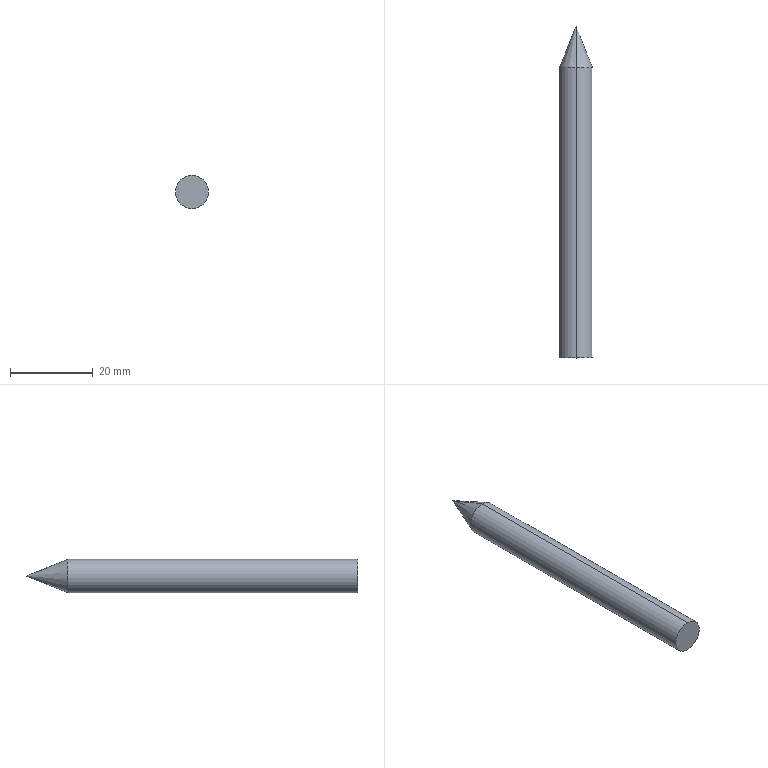Part | SolidWorks | features MirrorStock 1 | 1 solid | 5 faces | box 8 x 80 x 8 mm | volume 3686 mm3 | cone 2 | cylinder 2 | plane 1 | commonest cylinder face diameters 8 x2
STEP:
#1=CARTESIAN_POINT('',(0.,80.,0.));
#2=VERTEX_POINT('',#1);
#3=CARTESIAN_POINT('',(0.,70.,4.));
#4=VERTEX_POINT('',#3);
#5=CARTESIAN_POINT('',(0.,80.,0.));
#6=DIRECTION('',(0.,-0.9285,0.3714));
#7=VECTOR('',#6,1000.);
#8=LINE('',#5,#7);
#9=EDGE_CURVE('',#2,#4,#8,.T.);
#10=ORIENTED_EDGE('',*,*,#9,.F.);
#11=CARTESIAN_POINT('',(0.,70.,-4.));
#12=VERTEX_POINT('',#11);
#13=CARTESIAN_POINT('',(0.,80.,0.));
#14=DIRECTION('',(0.,-0.9285,-0.3714));
#15=VECTOR('',#14,1000.);
#16=LINE('',#13,#15);
#17=EDGE_CURVE('',#2,#12,#16,.T.);
#18=ORIENTED_EDGE('',*,*,#17,.T.);
#19=CARTESIAN_POINT('',(0.,70.,0.));
#20=DIRECTION('',(0.,1.,0.));
#21=DIRECTION('',(0.,0.,1.));
#22=AXIS2_PLACEMENT_3D('',#19,#20,#21);
#23=CIRCLE('',#22,4.);
#24=EDGE_CURVE('',#12,#4,#23,.T.);
#25=ORIENTED_EDGE('',*,*,#24,.T.);
#26=EDGE_LOOP('',(#10,#18,#25));
#27=FACE_OUTER_BOUND('',#26,.T.);
#28=CARTESIAN_POINT('',(0.,-920.,0.));
#29=DIRECTION('',(0.,-1.,0.));
#30=DIRECTION('',(0.,0.,1.));
#31=AXIS2_PLACEMENT_3D('',#28,#29,#30);
#32=CONICAL_SURFACE('',#31,400.,0.3805);
#33=ADVANCED_FACE('',(#27),#32,.T.);
#34=ORIENTED_EDGE('',*,*,#24,.F.);
#35=CARTESIAN_POINT('',(0.,0.,-4.));
#36=VERTEX_POINT('',#35);
#37=CARTESIAN_POINT('',(0.,0.,-4.));
#38=DIRECTION('',(0.,-1.,0.));
#39=VECTOR('',#38,1000.);
#40=LINE('',#37,#39);
#41=EDGE_CURVE('',#12,#36,#40,.T.);
#42=ORIENTED_EDGE('',*,*,#41,.T.);
#43=CARTESIAN_POINT('',(0.,0.,4.));
#44=VERTEX_POINT('',#43);
#45=CARTESIAN_POINT('',(0.,0.,0.));
#46=DIRECTION('',(0.,1.,0.));
#47=DIRECTION('',(0.,0.,1.));
#48=AXIS2_PLACEMENT_3D('',#45,#46,#47);
#49=CIRCLE('',#48,4.);
#50=EDGE_CURVE('',#36,#44,#49,.T.);
#51=ORIENTED_EDGE('',*,*,#50,.T.);
#52=CARTESIAN_POINT('',(0.,0.,4.));
#53=DIRECTION('',(0.,-1.,0.));
#54=VECTOR('',#53,1000.);
#55=LINE('',#52,#54);
#56=EDGE_CURVE('',#4,#44,#55,.T.);
#57=ORIENTED_EDGE('',*,*,#56,.F.);
#58=EDGE_LOOP('',(#34,#42,#51,#57));
#59=FACE_OUTER_BOUND('',#58,.T.);
#60=CARTESIAN_POINT('',(0.,0.,0.));
#61=DIRECTION('',(0.,-1.,0.));
#62=DIRECTION('',(0.,0.,1.));
#63=AXIS2_PLACEMENT_3D('',#60,#61,#62);
#64=CYLINDRICAL_SURFACE('',#63,4.);
#65=ADVANCED_FACE('',(#59),#64,.T.);
#66=CARTESIAN_POINT('',(0.,0.,0.));
#67=DIRECTION('',(0.,1.,0.));
#68=DIRECTION('',(0.,0.,1.));
#69=AXIS2_PLACEMENT_3D('',#66,#67,#68);
#70=CIRCLE('',#69,4.);
#71=EDGE_CURVE('',#44,#36,#70,.T.);
#72=ORIENTED_EDGE('',*,*,#71,.F.);
#73=ORIENTED_EDGE('',*,*,#50,.F.);
#74=EDGE_LOOP('',(#72,#73));
#75=FACE_OUTER_BOUND('',#74,.T.);
#76=CARTESIAN_POINT('',(0.,0.,0.));
#77=DIRECTION('',(0.,1.,0.));
#78=DIRECTION('',(0.,0.,-1.));
#79=AXIS2_PLACEMENT_3D('',#76,#77,#78);
#80=PLANE('',#79);
#81=ADVANCED_FACE('',(#75),#80,.F.);
#82=ORIENTED_EDGE('',*,*,#41,.F.);
#83=CARTESIAN_POINT('',(0.,70.,0.));
#84=DIRECTION('',(0.,1.,0.));
#85=DIRECTION('',(0.,0.,1.));
#86=AXIS2_PLACEMENT_3D('',#83,#84,#85);
#87=CIRCLE('',#86,4.);
#88=EDGE_CURVE('',#4,#12,#87,.T.);
#89=ORIENTED_EDGE('',*,*,#88,.F.);
#90=ORIENTED_EDGE('',*,*,#56,.T.);
#91=ORIENTED_EDGE('',*,*,#71,.T.);
#92=EDGE_LOOP('',(#82,#89,#90,#91));
#93=FACE_OUTER_BOUND('',#92,.T.);
#94=CARTESIAN_POINT('',(0.,0.,0.));
#95=DIRECTION('',(0.,-1.,0.));
#96=DIRECTION('',(0.,0.,1.));
#97=AXIS2_PLACEMENT_3D('',#94,#95,#96);
#98=CYLINDRICAL_SURFACE('',#97,4.);
#99=ADVANCED_FACE('',(#93),#98,.T.);
#100=ORIENTED_EDGE('',*,*,#17,.F.);
#101=ORIENTED_EDGE('',*,*,#9,.T.);
#102=ORIENTED_EDGE('',*,*,#88,.T.);
#103=EDGE_LOOP('',(#100,#101,#102));
#104=FACE_OUTER_BOUND('',#103,.T.);
#105=CARTESIAN_POINT('',(0.,-920.,0.));
#106=DIRECTION('',(0.,-1.,0.));
#107=DIRECTION('',(0.,0.,1.));
#108=AXIS2_PLACEMENT_3D('',#105,#106,#107);
#109=CONICAL_SURFACE('',#108,400.,0.3805);
#110=ADVANCED_FACE('',(#104),#109,.T.);
#111=CLOSED_SHELL('',(#33,#65,#81,#99,#110));
#112=MANIFOLD_SOLID_BREP('',#111);
#113=CARTESIAN_POINT('',(0.,0.,0.));
#114=DIRECTION('',(0.,0.,1.));
#115=DIRECTION('',(1.,0.,0.));
#116=AXIS2_PLACEMENT_3D('',#113,#114,#115);
#117=(LENGTH_UNIT()NAMED_UNIT(*)SI_UNIT(.MILLI.,.METRE.));
#118=UNCERTAINTY_MEASURE_WITH_UNIT(LENGTH_MEASURE(0.00001),#117,'','');
#119=(NAMED_UNIT(*)PLANE_ANGLE_UNIT()SI_UNIT($,.RADIAN.));
#120=(NAMED_UNIT(*)SI_UNIT($,.STERADIAN.)SOLID_ANGLE_UNIT());
#121=(GEOMETRIC_REPRESENTATION_CONTEXT(3)GLOBAL_UNCERTAINTY_ASSIGNED_CONTEXT((#118))GLOBAL_UNIT_ASSIGNED_CONTEXT((#117,#119,#120))REPRESENTATION_CONTEXT('',''));
#122=ADVANCED_BREP_SHAPE_REPRESENTATION('',(#112,#116),#121);